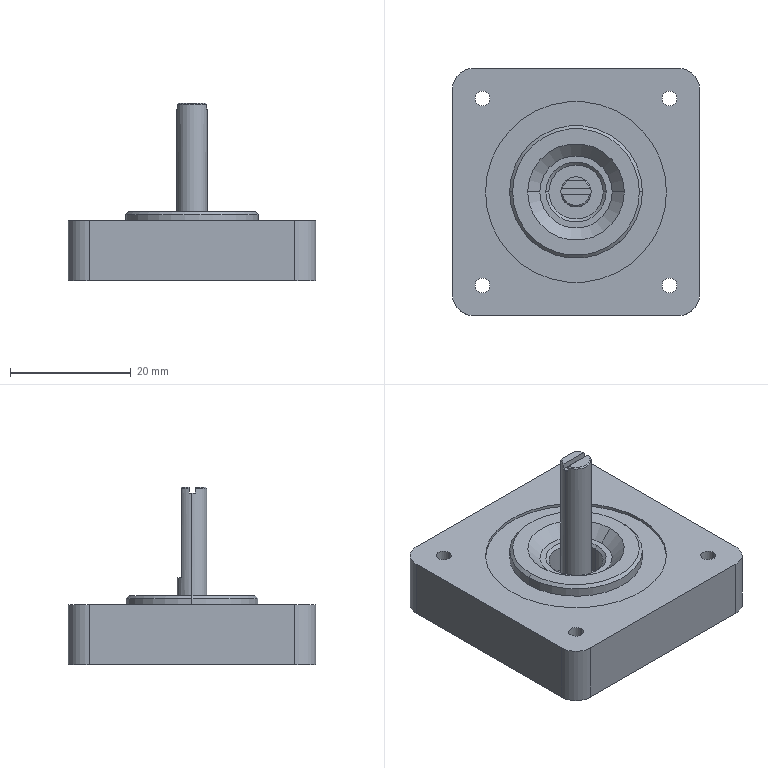Part | SolidWorks | features BaseBody 1 | 1 solid | 46 faces | box 41 x 41 x 29.5 mm | volume 16742 mm3 | cylinder 20 | plane 17 | cone 9 | commonest cylinder face diameters 2.459 x8 7 x4 5 x2 9 x2 22 x2 30 x2
STEP:
#1=CARTESIAN_POINT('',(-1.457,31.548,0.));
#2=VERTEX_POINT('',#1);
#3=CARTESIAN_POINT('',(-3.916,31.548,0.));
#4=VERTEX_POINT('',#3);
#5=CARTESIAN_POINT('',(-2.686,31.548,0.));
#6=DIRECTION('',(0.,0.,-1.));
#7=DIRECTION('',(1.,0.,0.));
#8=AXIS2_PLACEMENT_3D('',#5,#6,#7);
#9=CIRCLE('',#8,1.23);
#10=EDGE_CURVE('',#2,#4,#9,.T.);
#11=ORIENTED_EDGE('',*,*,#10,.T.);
#12=CARTESIAN_POINT('',(-3.916,31.548,10.));
#13=VERTEX_POINT('',#12);
#14=CARTESIAN_POINT('',(-3.916,31.548,-55.056));
#15=DIRECTION('',(0.,0.,1.));
#16=VECTOR('',#15,1000.);
#17=LINE('',#14,#16);
#18=EDGE_CURVE('',#4,#13,#17,.T.);
#19=ORIENTED_EDGE('',*,*,#18,.T.);
#20=CARTESIAN_POINT('',(-1.457,31.548,10.));
#21=VERTEX_POINT('',#20);
#22=CARTESIAN_POINT('',(-2.686,31.548,10.));
#23=DIRECTION('',(0.,0.,-1.));
#24=DIRECTION('',(1.,0.,0.));
#25=AXIS2_PLACEMENT_3D('',#22,#23,#24);
#26=CIRCLE('',#25,1.23);
#27=EDGE_CURVE('',#21,#13,#26,.T.);
#28=ORIENTED_EDGE('',*,*,#27,.F.);
#29=CARTESIAN_POINT('',(-1.457,31.548,-55.056));
#30=DIRECTION('',(0.,0.,1.));
#31=VECTOR('',#30,1000.);
#32=LINE('',#29,#31);
#33=EDGE_CURVE('',#2,#21,#32,.T.);
#34=ORIENTED_EDGE('',*,*,#33,.F.);
#35=EDGE_LOOP('',(#11,#19,#28,#34));
#36=FACE_OUTER_BOUND('',#35,.T.);
#37=CARTESIAN_POINT('',(-2.686,31.548,-55.056));
#38=DIRECTION('',(0.,0.,1.));
#39=DIRECTION('',(1.,0.,0.));
#40=AXIS2_PLACEMENT_3D('',#37,#38,#39);
#41=CYLINDRICAL_SURFACE('',#40,1.23);
#42=ADVANCED_FACE('',(#36),#41,.F.);
#43=CARTESIAN_POINT('',(-32.457,0.548,0.));
#44=VERTEX_POINT('',#43);
#45=CARTESIAN_POINT('',(-34.916,0.548,0.));
#46=VERTEX_POINT('',#45);
#47=CARTESIAN_POINT('',(-33.686,0.548,0.));
#48=DIRECTION('',(0.,0.,-1.));
#49=DIRECTION('',(1.,0.,0.));
#50=AXIS2_PLACEMENT_3D('',#47,#48,#49);
#51=CIRCLE('',#50,1.23);
#52=EDGE_CURVE('',#44,#46,#51,.T.);
#53=ORIENTED_EDGE('',*,*,#52,.T.);
#54=CARTESIAN_POINT('',(-34.916,0.548,10.));
#55=VERTEX_POINT('',#54);
#56=CARTESIAN_POINT('',(-34.916,0.548,-55.056));
#57=DIRECTION('',(0.,0.,1.));
#58=VECTOR('',#57,1000.);
#59=LINE('',#56,#58);
#60=EDGE_CURVE('',#46,#55,#59,.T.);
#61=ORIENTED_EDGE('',*,*,#60,.T.);
#62=CARTESIAN_POINT('',(-32.457,0.548,10.));
#63=VERTEX_POINT('',#62);
#64=CARTESIAN_POINT('',(-33.686,0.548,10.));
#65=DIRECTION('',(0.,0.,-1.));
#66=DIRECTION('',(1.,0.,0.));
#67=AXIS2_PLACEMENT_3D('',#64,#65,#66);
#68=CIRCLE('',#67,1.23);
#69=EDGE_CURVE('',#63,#55,#68,.T.);
#70=ORIENTED_EDGE('',*,*,#69,.F.);
#71=CARTESIAN_POINT('',(-32.457,0.548,-55.056));
#72=DIRECTION('',(0.,0.,1.));
#73=VECTOR('',#72,1000.);
#74=LINE('',#71,#73);
#75=EDGE_CURVE('',#44,#63,#74,.T.);
#76=ORIENTED_EDGE('',*,*,#75,.F.);
#77=EDGE_LOOP('',(#53,#61,#70,#76));
#78=FACE_OUTER_BOUND('',#77,.T.);
#79=CARTESIAN_POINT('',(-33.686,0.548,-55.056));
#80=DIRECTION('',(0.,0.,1.));
#81=DIRECTION('',(1.,0.,0.));
#82=AXIS2_PLACEMENT_3D('',#79,#80,#81);
#83=CYLINDRICAL_SURFACE('',#82,1.23);
#84=ADVANCED_FACE('',(#78),#83,.F.);
#85=CARTESIAN_POINT('',(-32.457,31.548,0.));
#86=VERTEX_POINT('',#85);
#87=CARTESIAN_POINT('',(-34.916,31.548,0.));
#88=VERTEX_POINT('',#87);
#89=CARTESIAN_POINT('',(-33.686,31.548,0.));
#90=DIRECTION('',(0.,0.,-1.));
#91=DIRECTION('',(1.,0.,0.));
#92=AXIS2_PLACEMENT_3D('',#89,#90,#91);
#93=CIRCLE('',#92,1.23);
#94=EDGE_CURVE('',#86,#88,#93,.T.);
#95=ORIENTED_EDGE('',*,*,#94,.T.);
#96=CARTESIAN_POINT('',(-34.916,31.548,10.));
#97=VERTEX_POINT('',#96);
#98=CARTESIAN_POINT('',(-34.916,31.548,-55.056));
#99=DIRECTION('',(0.,0.,1.));
#100=VECTOR('',#99,1000.);
#101=LINE('',#98,#100);
#102=EDGE_CURVE('',#88,#97,#101,.T.);
#103=ORIENTED_EDGE('',*,*,#102,.T.);
#104=CARTESIAN_POINT('',(-32.457,31.548,10.));
#105=VERTEX_POINT('',#104);
#106=CARTESIAN_POINT('',(-33.686,31.548,10.));
#107=DIRECTION('',(0.,0.,-1.));
#108=DIRECTION('',(1.,0.,0.));
#109=AXIS2_PLACEMENT_3D('',#106,#107,#108);
#110=CIRCLE('',#109,1.23);
#111=EDGE_CURVE('',#105,#97,#110,.T.);
#112=ORIENTED_EDGE('',*,*,#111,.F.);
#113=CARTESIAN_POINT('',(-32.457,31.548,-55.056));
#114=DIRECTION('',(0.,0.,1.));
#115=VECTOR('',#114,1000.);
#116=LINE('',#113,#115);
#117=EDGE_CURVE('',#86,#105,#116,.T.);
#118=ORIENTED_EDGE('',*,*,#117,.F.);
#119=EDGE_LOOP('',(#95,#103,#112,#118));
#120=FACE_OUTER_BOUND('',#119,.T.);
#121=CARTESIAN_POINT('',(-33.686,31.548,-55.056));
#122=DIRECTION('',(0.,0.,1.));
#123=DIRECTION('',(1.,0.,0.));
#124=AXIS2_PLACEMENT_3D('',#121,#122,#123);
#125=CYLINDRICAL_SURFACE('',#124,1.23);
#126=ADVANCED_FACE('',(#120),#125,.F.);
#127=CARTESIAN_POINT('',(-1.457,0.548,0.));
#128=VERTEX_POINT('',#127);
#129=CARTESIAN_POINT('',(-3.916,0.548,0.));
#130=VERTEX_POINT('',#129);
#131=CARTESIAN_POINT('',(-2.686,0.548,0.));
#132=DIRECTION('',(0.,0.,-1.));
#133=DIRECTION('',(1.,0.,0.));
#134=AXIS2_PLACEMENT_3D('',#131,#132,#133);
#135=CIRCLE('',#134,1.23);
#136=EDGE_CURVE('',#128,#130,#135,.T.);
#137=ORIENTED_EDGE('',*,*,#136,.T.);
#138=CARTESIAN_POINT('',(-3.916,0.548,10.));
#139=VERTEX_POINT('',#138);
#140=CARTESIAN_POINT('',(-3.916,0.548,-55.056));
#141=DIRECTION('',(0.,0.,1.));
#142=VECTOR('',#141,1000.);
#143=LINE('',#140,#142);
#144=EDGE_CURVE('',#130,#139,#143,.T.);
#145=ORIENTED_EDGE('',*,*,#144,.T.);
#146=CARTESIAN_POINT('',(-1.457,0.548,10.));
#147=VERTEX_POINT('',#146);
#148=CARTESIAN_POINT('',(-2.686,0.548,10.));
#149=DIRECTION('',(0.,0.,-1.));
#150=DIRECTION('',(1.,0.,0.));
#151=AXIS2_PLACEMENT_3D('',#148,#149,#150);
#152=CIRCLE('',#151,1.23);
#153=EDGE_CURVE('',#147,#139,#152,.T.);
#154=ORIENTED_EDGE('',*,*,#153,.F.);
#155=CARTESIAN_POINT('',(-1.457,0.548,-55.056));
#156=DIRECTION('',(0.,0.,1.));
#157=VECTOR('',#156,1000.);
#158=LINE('',#155,#157);
#159=EDGE_CURVE('',#128,#147,#158,.T.);
#160=ORIENTED_EDGE('',*,*,#159,.F.);
#161=EDGE_LOOP('',(#137,#145,#154,#160));
#162=FACE_OUTER_BOUND('',#161,.T.);
#163=CARTESIAN_POINT('',(-2.686,0.548,-55.056));
#164=DIRECTION('',(0.,0.,1.));
#165=DIRECTION('',(1.,0.,0.));
#166=AXIS2_PLACEMENT_3D('',#163,#164,#165);
#167=CYLINDRICAL_SURFACE('',#166,1.23);
#168=ADVANCED_FACE('',(#162),#167,.F.);
#169=CARTESIAN_POINT('',(-3.186,16.048,10.));
#170=VERTEX_POINT('',#169);
#171=CARTESIAN_POINT('',(-33.186,16.048,10.));
#172=VERTEX_POINT('',#171);
#173=CARTESIAN_POINT('',(-18.186,16.048,10.));
#174=DIRECTION('',(0.,0.,-1.));
#175=DIRECTION('',(-1.,0.,0.));
#176=AXIS2_PLACEMENT_3D('',#173,#174,#175);
#177=CIRCLE('',#176,15.);
#178=EDGE_CURVE('',#170,#172,#177,.T.);
#179=ORIENTED_EDGE('',*,*,#178,.F.);
#180=CARTESIAN_POINT('',(-3.186,16.048,9.5));
#181=VERTEX_POINT('',#180);
#182=CARTESIAN_POINT('',(-3.186,16.048,10.));
#183=DIRECTION('',(0.,0.,-1.));
#184=VECTOR('',#183,1000.);
#185=LINE('',#182,#184);
#186=EDGE_CURVE('',#170,#181,#185,.T.);
#187=ORIENTED_EDGE('',*,*,#186,.T.);
#188=CARTESIAN_POINT('',(-33.186,16.048,9.5));
#189=VERTEX_POINT('',#188);
#190=CARTESIAN_POINT('',(-18.186,16.048,9.5));
#191=DIRECTION('',(0.,0.,1.));
#192=DIRECTION('',(-1.,0.,0.));
#193=AXIS2_PLACEMENT_3D('',#190,#191,#192);
#194=CIRCLE('',#193,15.);
#195=EDGE_CURVE('',#189,#181,#194,.T.);
#196=ORIENTED_EDGE('',*,*,#195,.F.);
#197=CARTESIAN_POINT('',(-33.186,16.048,10.));
#198=DIRECTION('',(0.,0.,-1.));
#199=VECTOR('',#198,1000.);
#200=LINE('',#197,#199);
#201=EDGE_CURVE('',#172,#189,#200,.T.);
#202=ORIENTED_EDGE('',*,*,#201,.F.);
#203=EDGE_LOOP('',(#179,#187,#196,#202));
#204=FACE_OUTER_BOUND('',#203,.T.);
#205=CARTESIAN_POINT('',(-18.186,16.048,10.));
#206=DIRECTION('',(0.,0.,-1.));
#207=DIRECTION('',(-1.,0.,0.));
#208=AXIS2_PLACEMENT_3D('',#205,#206,#207);
#209=CYLINDRICAL_SURFACE('',#208,15.);
#210=ADVANCED_FACE('',(#204),#209,.F.);
#211=CARTESIAN_POINT('',(-7.186,16.048,9.5));
#212=VERTEX_POINT('',#211);
#213=CARTESIAN_POINT('',(-29.186,16.048,9.5));
#214=VERTEX_POINT('',#213);
#215=CARTESIAN_POINT('',(-18.186,16.048,9.5));
#216=DIRECTION('',(0.,0.,1.));
#217=DIRECTION('',(1.,0.,0.));
#218=AXIS2_PLACEMENT_3D('',#215,#216,#217);
#219=CIRCLE('',#218,11.);
#220=EDGE_CURVE('',#212,#214,#219,.T.);
#221=ORIENTED_EDGE('',*,*,#220,.T.);
#222=CARTESIAN_POINT('',(-29.186,16.048,11.));
#223=VERTEX_POINT('',#222);
#224=CARTESIAN_POINT('',(-29.186,16.048,9.5));
#225=DIRECTION('',(0.,0.,1.));
#226=VECTOR('',#225,1000.);
#227=LINE('',#224,#226);
#228=EDGE_CURVE('',#214,#223,#227,.T.);
#229=ORIENTED_EDGE('',*,*,#228,.T.);
#230=CARTESIAN_POINT('',(-7.186,16.048,11.));
#231=VERTEX_POINT('',#230);
#232=CARTESIAN_POINT('',(-18.186,16.048,11.));
#233=DIRECTION('',(0.,0.,-1.));
#234=DIRECTION('',(1.,0.,0.));
#235=AXIS2_PLACEMENT_3D('',#232,#233,#234);
#236=CIRCLE('',#235,11.);
#237=EDGE_CURVE('',#223,#231,#236,.T.);
#238=ORIENTED_EDGE('',*,*,#237,.T.);
#239=CARTESIAN_POINT('',(-7.186,16.048,9.5));
#240=DIRECTION('',(0.,0.,1.));
#241=VECTOR('',#240,1000.);
#242=LINE('',#239,#241);
#243=EDGE_CURVE('',#212,#231,#242,.T.);
#244=ORIENTED_EDGE('',*,*,#243,.F.);
#245=EDGE_LOOP('',(#221,#229,#238,#244));
#246=FACE_OUTER_BOUND('',#245,.T.);
#247=CARTESIAN_POINT('',(-18.186,16.048,9.5));
#248=DIRECTION('',(0.,0.,1.));
#249=DIRECTION('',(1.,0.,0.));
#250=AXIS2_PLACEMENT_3D('',#247,#248,#249);
#251=CYLINDRICAL_SURFACE('',#250,11.);
#252=ADVANCED_FACE('',(#246),#251,.T.);
#253=CARTESIAN_POINT('',(-28.686,16.048,11.5));
#254=VERTEX_POINT('',#253);
#255=CARTESIAN_POINT('',(-7.686,16.048,11.5));
#256=VERTEX_POINT('',#255);
#257=CARTESIAN_POINT('',(-18.186,16.048,11.5));
#258=DIRECTION('',(0.,0.,-1.));
#259=DIRECTION('',(-1.,0.,0.));
#260=AXIS2_PLACEMENT_3D('',#257,#258,#259);
#261=CIRCLE('',#260,10.5);
#262=EDGE_CURVE('',#254,#256,#261,.T.);
#263=ORIENTED_EDGE('',*,*,#262,.T.);
#264=CARTESIAN_POINT('',(-7.186,16.048,11.));
#265=DIRECTION('',(0.7071,0.,-0.7071));
#266=VECTOR('',#265,1000.);
#267=LINE('',#264,#266);
#268=EDGE_CURVE('',#256,#231,#267,.T.);
#269=ORIENTED_EDGE('',*,*,#268,.T.);
#270=ORIENTED_EDGE('',*,*,#237,.F.);
#271=CARTESIAN_POINT('',(-29.186,16.048,11.));
#272=DIRECTION('',(-0.7071,0.,-0.7071));
#273=VECTOR('',#272,1000.);
#274=LINE('',#271,#273);
#275=EDGE_CURVE('',#254,#223,#274,.T.);
#276=ORIENTED_EDGE('',*,*,#275,.F.);
#277=EDGE_LOOP('',(#263,#269,#270,#276));
#278=FACE_OUTER_BOUND('',#277,.T.);
#279=CARTESIAN_POINT('',(-18.186,16.048,11.));
#280=DIRECTION('',(0.,0.,-1.));
#281=DIRECTION('',(-1.,0.,0.));
#282=AXIS2_PLACEMENT_3D('',#279,#280,#281);
#283=CONICAL_SURFACE('',#282,11.,0.7854);
#284=ADVANCED_FACE('',(#278),#283,.T.);
#285=CARTESIAN_POINT('',(-24.186,16.048,9.5));
#286=VERTEX_POINT('',#285);
#287=CARTESIAN_POINT('',(-12.186,16.048,9.5));
#288=VERTEX_POINT('',#287);
#289=CARTESIAN_POINT('',(-18.186,16.048,9.5));
#290=DIRECTION('',(0.,0.,1.));
#291=DIRECTION('',(1.,0.,0.));
#292=AXIS2_PLACEMENT_3D('',#289,#290,#291);
#293=CIRCLE('',#292,6.);
#294=EDGE_CURVE('',#286,#288,#293,.T.);
#295=ORIENTED_EDGE('',*,*,#294,.F.);
#296=CARTESIAN_POINT('',(-26.186,16.048,11.5));
#297=VERTEX_POINT('',#296);
#298=CARTESIAN_POINT('',(-26.186,16.048,11.5));
#299=DIRECTION('',(-0.7071,0.,0.7071));
#300=VECTOR('',#299,1000.);
#301=LINE('',#298,#300);
#302=EDGE_CURVE('',#286,#297,#301,.T.);
#303=ORIENTED_EDGE('',*,*,#302,.T.);
#304=CARTESIAN_POINT('',(-10.186,16.048,11.5));
#305=VERTEX_POINT('',#304);
#306=CARTESIAN_POINT('',(-18.186,16.048,11.5));
#307=DIRECTION('',(0.,0.,1.));
#308=DIRECTION('',(1.,0.,0.));
#309=AXIS2_PLACEMENT_3D('',#306,#307,#308);
#310=CIRCLE('',#309,8.);
#311=EDGE_CURVE('',#297,#305,#310,.T.);
#312=ORIENTED_EDGE('',*,*,#311,.T.);
#313=CARTESIAN_POINT('',(-10.186,16.048,11.5));
#314=DIRECTION('',(0.7071,0.,0.7071));
#315=VECTOR('',#314,1000.);
#316=LINE('',#313,#315);
#317=EDGE_CURVE('',#288,#305,#316,.T.);
#318=ORIENTED_EDGE('',*,*,#317,.F.);
#319=EDGE_LOOP('',(#295,#303,#312,#318));
#320=FACE_OUTER_BOUND('',#319,.T.);
#321=CARTESIAN_POINT('',(-18.186,16.048,11.5));
#322=DIRECTION('',(0.,0.,1.));
#323=DIRECTION('',(1.,0.,0.));
#324=AXIS2_PLACEMENT_3D('',#321,#322,#323);
#325=CONICAL_SURFACE('',#324,8.,0.7854);
#326=ADVANCED_FACE('',(#320),#325,.F.);
#327=CARTESIAN_POINT('',(-22.686,16.048,9.));
#328=VERTEX_POINT('',#327);
#329=CARTESIAN_POINT('',(-13.686,16.048,9.));
#330=VERTEX_POINT('',#329);
#331=CARTESIAN_POINT('',(-18.186,16.048,9.));
#332=DIRECTION('',(0.,0.,1.));
#333=DIRECTION('',(-1.,0.,0.));
#334=AXIS2_PLACEMENT_3D('',#331,#332,#333);
#335=CIRCLE('',#334,4.5);
#336=EDGE_CURVE('',#328,#330,#335,.T.);
#337=ORIENTED_EDGE('',*,*,#336,.F.);
#338=CARTESIAN_POINT('',(-23.186,16.048,9.5));
#339=VERTEX_POINT('',#338);
#340=CARTESIAN_POINT('',(-23.186,16.048,9.5));
#341=DIRECTION('',(-0.7071,0.,0.7071));
#342=VECTOR('',#341,1000.);
#343=LINE('',#340,#342);
#344=EDGE_CURVE('',#328,#339,#343,.T.);
#345=ORIENTED_EDGE('',*,*,#344,.T.);
#346=CARTESIAN_POINT('',(-13.186,16.048,9.5));
#347=VERTEX_POINT('',#346);
#348=CARTESIAN_POINT('',(-18.186,16.048,9.5));
#349=DIRECTION('',(0.,0.,1.));
#350=DIRECTION('',(1.,0.,0.));
#351=AXIS2_PLACEMENT_3D('',#348,#349,#350);
#352=CIRCLE('',#351,5.);
#353=EDGE_CURVE('',#339,#347,#352,.T.);
#354=ORIENTED_EDGE('',*,*,#353,.T.);
#355=CARTESIAN_POINT('',(-13.186,16.048,9.5));
#356=DIRECTION('',(0.7071,0.,0.7071));
#357=VECTOR('',#356,1000.);
#358=LINE('',#355,#357);
#359=EDGE_CURVE('',#330,#347,#358,.T.);
#360=ORIENTED_EDGE('',*,*,#359,.F.);
#361=EDGE_LOOP('',(#337,#345,#354,#360));
#362=FACE_OUTER_BOUND('',#361,.T.);
#363=CARTESIAN_POINT('',(-18.186,16.048,9.5));
#364=DIRECTION('',(0.,0.,1.));
#365=DIRECTION('',(1.,0.,0.));
#366=AXIS2_PLACEMENT_3D('',#363,#364,#365);
#367=CONICAL_SURFACE('',#366,5.,0.7854);
#368=ADVANCED_FACE('',(#362),#367,.F.);
#369=CARTESIAN_POINT('',(-22.686,16.048,4.5));
#370=VERTEX_POINT('',#369);
#371=CARTESIAN_POINT('',(-13.686,16.048,4.5));
#372=VERTEX_POINT('',#371);
#373=CARTESIAN_POINT('',(-18.186,16.048,4.5));
#374=DIRECTION('',(0.,0.,1.));
#375=DIRECTION('',(1.,0.,0.));
#376=AXIS2_PLACEMENT_3D('',#373,#374,#375);
#377=CIRCLE('',#376,4.5);
#378=EDGE_CURVE('',#370,#372,#377,.T.);
#379=ORIENTED_EDGE('',*,*,#378,.F.);
#380=CARTESIAN_POINT('',(-22.686,16.048,7.));
#381=DIRECTION('',(0.,0.,1.));
#382=VECTOR('',#381,1000.);
#383=LINE('',#380,#382);
#384=EDGE_CURVE('',#370,#328,#383,.T.);
#385=ORIENTED_EDGE('',*,*,#384,.T.);
#386=ORIENTED_EDGE('',*,*,#336,.T.);
#387=CARTESIAN_POINT('',(-13.686,16.048,7.));
#388=DIRECTION('',(0.,0.,1.));
#389=VECTOR('',#388,1000.);
#390=LINE('',#387,#389);
#391=EDGE_CURVE('',#372,#330,#390,.T.);
#392=ORIENTED_EDGE('',*,*,#391,.F.);
#393=EDGE_LOOP('',(#379,#385,#386,#392));
#394=FACE_OUTER_BOUND('',#393,.T.);
#395=CARTESIAN_POINT('',(-18.186,16.048,7.));
#396=DIRECTION('',(0.,0.,1.));
#397=DIRECTION('',(1.,0.,0.));
#398=AXIS2_PLACEMENT_3D('',#395,#396,#397);
#399=CYLINDRICAL_SURFACE('',#398,4.5);
#400=ADVANCED_FACE('',(#394),#399,.F.);
#401=CARTESIAN_POINT('',(-20.686,16.048,4.5));
#402=VERTEX_POINT('',#401);
#403=CARTESIAN_POINT('',(-15.686,16.048,4.5));
#404=VERTEX_POINT('',#403);
#405=CARTESIAN_POINT('',(-18.186,16.048,4.5));
#406=DIRECTION('',(0.,0.,-1.));
#407=DIRECTION('',(1.,0.,0.));
#408=AXIS2_PLACEMENT_3D('',#405,#406,#407);
#409=CIRCLE('',#408,2.5);
#410=EDGE_CURVE('',#402,#404,#409,.T.);
#411=ORIENTED_EDGE('',*,*,#410,.F.);
#412=CARTESIAN_POINT('',(-20.686,16.048,28.5));
#413=VERTEX_POINT('',#412);
#414=CARTESIAN_POINT('',(-20.686,16.048,4.5));
#415=DIRECTION('',(0.,0.,1.));
#416=VECTOR('',#415,1000.);
#417=LINE('',#414,#416);
#418=EDGE_CURVE('',#402,#413,#417,.T.);
#419=ORIENTED_EDGE('',*,*,#418,.T.);
#420=CARTESIAN_POINT('',(-20.637,16.545,28.5));
#421=VERTEX_POINT('',#420);
#422=CARTESIAN_POINT('',(-18.186,16.048,28.5));
#423=DIRECTION('',(0.,0.,1.));
#424=DIRECTION('',(1.,0.,0.));
#425=AXIS2_PLACEMENT_3D('',#422,#423,#424);
#426=CIRCLE('',#425,2.5);
#427=EDGE_CURVE('',#421,#413,#426,.T.);
#428=ORIENTED_EDGE('',*,*,#427,.F.);
#429=CARTESIAN_POINT('',(-20.637,16.545,29.3));
#430=VERTEX_POINT('',#429);
#431=CARTESIAN_POINT('',(-20.637,16.545,29.5));
#432=DIRECTION('',(0.,0.,1.));
#433=VECTOR('',#432,1000.);
#434=LINE('',#431,#433);
#435=EDGE_CURVE('',#421,#430,#434,.T.);
#436=ORIENTED_EDGE('',*,*,#435,.T.);
#437=CARTESIAN_POINT('',(-19.921,17.848,29.3));
#438=VERTEX_POINT('',#437);
#439=CARTESIAN_POINT('',(-18.186,16.048,29.3));
#440=DIRECTION('',(0.,0.,-1.));
#441=DIRECTION('',(1.,0.,0.));
#442=AXIS2_PLACEMENT_3D('',#439,#440,#441);
#443=CIRCLE('',#442,2.5);
#444=EDGE_CURVE('',#430,#438,#443,.T.);
#445=ORIENTED_EDGE('',*,*,#444,.T.);
#446=CARTESIAN_POINT('',(-19.921,17.848,14.5));
#447=VERTEX_POINT('',#446);
#448=CARTESIAN_POINT('',(-19.921,17.848,4.5));
#449=DIRECTION('',(0.,0.,-1.));
#450=VECTOR('',#449,1000.);
#451=LINE('',#448,#450);
#452=EDGE_CURVE('',#438,#447,#451,.T.);
#453=ORIENTED_EDGE('',*,*,#452,.T.);
#454=CARTESIAN_POINT('',(-16.451,17.848,14.5));
#455=VERTEX_POINT('',#454);
#456=CARTESIAN_POINT('',(-18.186,16.048,14.5));
#457=DIRECTION('',(0.,0.,-1.));
#458=DIRECTION('',(1.,0.,0.));
#459=AXIS2_PLACEMENT_3D('',#456,#457,#458);
#460=CIRCLE('',#459,2.5);
#461=EDGE_CURVE('',#447,#455,#460,.T.);
#462=ORIENTED_EDGE('',*,*,#461,.T.);
#463=CARTESIAN_POINT('',(-16.451,17.848,29.3));
#464=VERTEX_POINT('',#463);
#465=CARTESIAN_POINT('',(-16.451,17.848,4.5));
#466=DIRECTION('',(0.,0.,1.));
#467=VECTOR('',#466,1000.);
#468=LINE('',#465,#467);
#469=EDGE_CURVE('',#455,#464,#468,.T.);
#470=ORIENTED_EDGE('',*,*,#469,.T.);
#471=CARTESIAN_POINT('',(-15.736,16.545,29.3));
#472=VERTEX_POINT('',#471);
#473=CARTESIAN_POINT('',(-18.186,16.048,29.3));
#474=DIRECTION('',(0.,0.,-1.));
#475=DIRECTION('',(1.,0.,0.));
#476=AXIS2_PLACEMENT_3D('',#473,#474,#475);
#477=CIRCLE('',#476,2.5);
#478=EDGE_CURVE('',#464,#472,#477,.T.);
#479=ORIENTED_EDGE('',*,*,#478,.T.);
#480=CARTESIAN_POINT('',(-15.736,16.545,28.5));
#481=VERTEX_POINT('',#480);
#482=CARTESIAN_POINT('',(-15.736,16.545,29.5));
#483=DIRECTION('',(0.,0.,-1.));
#484=VECTOR('',#483,1000.);
#485=LINE('',#482,#484);
#486=EDGE_CURVE('',#472,#481,#485,.T.);
#487=ORIENTED_EDGE('',*,*,#486,.T.);
#488=CARTESIAN_POINT('',(-15.686,16.048,28.5));
#489=VERTEX_POINT('',#488);
#490=CARTESIAN_POINT('',(-18.186,16.048,28.5));
#491=DIRECTION('',(0.,0.,1.));
#492=DIRECTION('',(1.,0.,0.));
#493=AXIS2_PLACEMENT_3D('',#490,#491,#492);
#494=CIRCLE('',#493,2.5);
#495=EDGE_CURVE('',#489,#481,#494,.T.);
#496=ORIENTED_EDGE('',*,*,#495,.F.);
#497=CARTESIAN_POINT('',(-15.686,16.048,4.5));
#498=DIRECTION('',(0.,0.,1.));
#499=VECTOR('',#498,1000.);
#500=LINE('',#497,#499);
#501=EDGE_CURVE('',#404,#489,#500,.T.);
#502=ORIENTED_EDGE('',*,*,#501,.F.);
#503=EDGE_LOOP('',(#411,#419,#428,#436,#445,#453,#462,#470,#479,#487,#496,#502));
#504=FACE_OUTER_BOUND('',#503,.T.);
#505=CARTESIAN_POINT('',(-18.186,16.048,4.5));
#506=DIRECTION('',(0.,0.,1.));
#507=DIRECTION('',(1.,0.,0.));
#508=AXIS2_PLACEMENT_3D('',#505,#506,#507);
#509=CYLINDRICAL_SURFACE('',#508,2.5);
#510=ADVANCED_FACE('',(#504),#509,.T.);
#511=ORIENTED_EDGE('',*,*,#10,.F.);
#512=CARTESIAN_POINT('',(-2.686,31.548,0.));
#513=DIRECTION('',(0.,0.,-1.));
#514=DIRECTION('',(1.,0.,0.));
#515=AXIS2_PLACEMENT_3D('',#512,#513,#514);
#516=CIRCLE('',#515,1.23);
#517=EDGE_CURVE('',#4,#2,#516,.T.);
#518=ORIENTED_EDGE('',*,*,#517,.F.);
#519=EDGE_LOOP('',(#511,#518));
#520=FACE_BOUND('',#519,.T.);
#521=ORIENTED_EDGE('',*,*,#52,.F.);
#522=CARTESIAN_POINT('',(-33.686,0.548,0.));
#523=DIRECTION('',(0.,0.,-1.));
#524=DIRECTION('',(1.,0.,0.));
#525=AXIS2_PLACEMENT_3D('',#522,#523,#524);
#526=CIRCLE('',#525,1.23);
#527=EDGE_CURVE('',#46,#44,#526,.T.);
#528=ORIENTED_EDGE('',*,*,#527,.F.);
#529=EDGE_LOOP('',(#521,#528));
#530=FACE_BOUND('',#529,.T.);
#531=ORIENTED_EDGE('',*,*,#94,.F.);
#532=CARTESIAN_POINT('',(-33.686,31.548,0.));
#533=DIRECTION('',(0.,0.,-1.));
#534=DIRECTION('',(1.,0.,0.));
#535=AXIS2_PLACEMENT_3D('',#532,#533,#534);
#536=CIRCLE('',#535,1.23);
#537=EDGE_CURVE('',#88,#86,#536,.T.);
#538=ORIENTED_EDGE('',*,*,#537,.F.);
#539=EDGE_LOOP('',(#531,#538));
#540=FACE_BOUND('',#539,.T.);
#541=ORIENTED_EDGE('',*,*,#136,.F.);
#542=CARTESIAN_POINT('',(-2.686,0.548,0.));
#543=DIRECTION('',(0.,0.,-1.));
#544=DIRECTION('',(1.,0.,0.));
#545=AXIS2_PLACEMENT_3D('',#542,#543,#544);
#546=CIRCLE('',#545,1.23);
#547=EDGE_CURVE('',#130,#128,#546,.T.);
#548=ORIENTED_EDGE('',*,*,#547,.F.);
#549=EDGE_LOOP('',(#541,#548));
#550=FACE_BOUND('',#549,.T.);
#551=CARTESIAN_POINT('',(-38.686,33.048,0.));
#552=VERTEX_POINT('',#551);
#553=CARTESIAN_POINT('',(-38.686,-0.952,0.));
#554=VERTEX_POINT('',#553);
#555=CARTESIAN_POINT('',(-38.686,16.048,0.));
#556=DIRECTION('',(0.,-1.,0.));
#557=VECTOR('',#556,1000.);
#558=LINE('',#555,#557);
#559=EDGE_CURVE('',#552,#554,#558,.T.);
#560=ORIENTED_EDGE('',*,*,#559,.F.);
#561=CARTESIAN_POINT('',(-35.186,36.548,0.));
#562=VERTEX_POINT('',#561);
#563=CARTESIAN_POINT('',(-35.186,33.048,0.));
#564=DIRECTION('',(0.,0.,1.));
#565=DIRECTION('',(1.,0.,0.));
#566=AXIS2_PLACEMENT_3D('',#563,#564,#565);
#567=CIRCLE('',#566,3.5);
#568=EDGE_CURVE('',#562,#552,#567,.T.);
#569=ORIENTED_EDGE('',*,*,#568,.F.);
#570=CARTESIAN_POINT('',(-1.186,36.548,0.));
#571=VERTEX_POINT('',#570);
#572=CARTESIAN_POINT('',(-18.186,36.548,0.));
#573=DIRECTION('',(-1.,0.,0.));
#574=VECTOR('',#573,1000.);
#575=LINE('',#572,#574);
#576=EDGE_CURVE('',#571,#562,#575,.T.);
#577=ORIENTED_EDGE('',*,*,#576,.F.);
#578=CARTESIAN_POINT('',(2.314,33.048,0.));
#579=VERTEX_POINT('',#578);
#580=CARTESIAN_POINT('',(-1.186,33.048,0.));
#581=DIRECTION('',(0.,0.,1.));
#582=DIRECTION('',(1.,0.,0.));
#583=AXIS2_PLACEMENT_3D('',#580,#581,#582);
#584=CIRCLE('',#583,3.5);
#585=EDGE_CURVE('',#579,#571,#584,.T.);
#586=ORIENTED_EDGE('',*,*,#585,.F.);
#587=CARTESIAN_POINT('',(2.314,-0.952,0.));
#588=VERTEX_POINT('',#587);
#589=CARTESIAN_POINT('',(2.314,16.048,0.));
#590=DIRECTION('',(0.,1.,0.));
#591=VECTOR('',#590,1000.);
#592=LINE('',#589,#591);
#593=EDGE_CURVE('',#588,#579,#592,.T.);
#594=ORIENTED_EDGE('',*,*,#593,.F.);
#595=CARTESIAN_POINT('',(-1.186,-4.452,0.));
#596=VERTEX_POINT('',#595);
#597=CARTESIAN_POINT('',(-1.186,-0.952,0.));
#598=DIRECTION('',(0.,0.,1.));
#599=DIRECTION('',(1.,0.,0.));
#600=AXIS2_PLACEMENT_3D('',#597,#598,#599);
#601=CIRCLE('',#600,3.5);
#602=EDGE_CURVE('',#596,#588,#601,.T.);
#603=ORIENTED_EDGE('',*,*,#602,.F.);
#604=CARTESIAN_POINT('',(-35.186,-4.452,0.));
#605=VERTEX_POINT('',#604);
#606=CARTESIAN_POINT('',(-18.186,-4.452,0.));
#607=DIRECTION('',(1.,0.,0.));
#608=VECTOR('',#607,1000.);
#609=LINE('',#606,#608);
#610=EDGE_CURVE('',#605,#596,#609,.T.);
#611=ORIENTED_EDGE('',*,*,#610,.F.);
#612=CARTESIAN_POINT('',(-35.186,-0.952,0.));
#613=DIRECTION('',(0.,0.,1.));
#614=DIRECTION('',(1.,0.,0.));
#615=AXIS2_PLACEMENT_3D('',#612,#613,#614);
#616=CIRCLE('',#615,3.5);
#617=EDGE_CURVE('',#554,#605,#616,.T.);
#618=ORIENTED_EDGE('',*,*,#617,.F.);
#619=EDGE_LOOP('',(#560,#569,#577,#586,#594,#603,#611,#618));
#620=FACE_OUTER_BOUND('',#619,.T.);
#621=CARTESIAN_POINT('',(-18.186,16.048,0.));
#622=DIRECTION('',(0.,0.,1.));
#623=DIRECTION('',(1.,0.,0.));
#624=AXIS2_PLACEMENT_3D('',#621,#622,#623);
#625=PLANE('',#624);
#626=ADVANCED_FACE('',(#520,#530,#540,#550,#620),#625,.F.);
#627=ORIENTED_EDGE('',*,*,#18,.F.);
#628=ORIENTED_EDGE('',*,*,#517,.T.);
#629=ORIENTED_EDGE('',*,*,#33,.T.);
#630=CARTESIAN_POINT('',(-2.686,31.548,10.));
#631=DIRECTION('',(0.,0.,-1.));
#632=DIRECTION('',(1.,0.,0.));
#633=AXIS2_PLACEMENT_3D('',#630,#631,#632);
#634=CIRCLE('',#633,1.23);
#635=EDGE_CURVE('',#13,#21,#634,.T.);
#636=ORIENTED_EDGE('',*,*,#635,.F.);
#637=EDGE_LOOP('',(#627,#628,#629,#636));
#638=FACE_OUTER_BOUND('',#637,.T.);
#639=CARTESIAN_POINT('',(-2.686,31.548,-55.056));
#640=DIRECTION('',(0.,0.,1.));
#641=DIRECTION('',(1.,0.,0.));
#642=AXIS2_PLACEMENT_3D('',#639,#640,#641);
#643=CYLINDRICAL_SURFACE('',#642,1.23);
#644=ADVANCED_FACE('',(#638),#643,.F.);
#645=ORIENTED_EDGE('',*,*,#60,.F.);
#646=ORIENTED_EDGE('',*,*,#527,.T.);
#647=ORIENTED_EDGE('',*,*,#75,.T.);
#648=CARTESIAN_POINT('',(-33.686,0.548,10.));
#649=DIRECTION('',(0.,0.,-1.));
#650=DIRECTION('',(1.,0.,0.));
#651=AXIS2_PLACEMENT_3D('',#648,#649,#650);
#652=CIRCLE('',#651,1.23);
#653=EDGE_CURVE('',#55,#63,#652,.T.);
#654=ORIENTED_EDGE('',*,*,#653,.F.);
#655=EDGE_LOOP('',(#645,#646,#647,#654));
#656=FACE_OUTER_BOUND('',#655,.T.);
#657=CARTESIAN_POINT('',(-33.686,0.548,-55.056));
#658=DIRECTION('',(0.,0.,1.));
#659=DIRECTION('',(1.,0.,0.));
#660=AXIS2_PLACEMENT_3D('',#657,#658,#659);
#661=CYLINDRICAL_SURFACE('',#660,1.23);
#662=ADVANCED_FACE('',(#656),#661,.F.);
#663=ORIENTED_EDGE('',*,*,#102,.F.);
#664=ORIENTED_EDGE('',*,*,#537,.T.);
#665=ORIENTED_EDGE('',*,*,#117,.T.);
#666=CARTESIAN_POINT('',(-33.686,31.548,10.));
#667=DIRECTION('',(0.,0.,-1.));
#668=DIRECTION('',(1.,0.,0.));
#669=AXIS2_PLACEMENT_3D('',#666,#667,#668);
#670=CIRCLE('',#669,1.23);
#671=EDGE_CURVE('',#97,#105,#670,.T.);
#672=ORIENTED_EDGE('',*,*,#671,.F.);
#673=EDGE_LOOP('',(#663,#664,#665,#672));
#674=FACE_OUTER_BOUND('',#673,.T.);
#675=CARTESIAN_POINT('',(-33.686,31.548,-55.056));
#676=DIRECTION('',(0.,0.,1.));
#677=DIRECTION('',(1.,0.,0.));
#678=AXIS2_PLACEMENT_3D('',#675,#676,#677);
#679=CYLINDRICAL_SURFACE('',#678,1.23);
#680=ADVANCED_FACE('',(#674),#679,.F.);
#681=ORIENTED_EDGE('',*,*,#144,.F.);
#682=ORIENTED_EDGE('',*,*,#547,.T.);
#683=ORIENTED_EDGE('',*,*,#159,.T.);
#684=CARTESIAN_POINT('',(-2.686,0.548,10.));
#685=DIRECTION('',(0.,0.,-1.));
#686=DIRECTION('',(1.,0.,0.));
#687=AXIS2_PLACEMENT_3D('',#684,#685,#686);
#688=CIRCLE('',#687,1.23);
#689=EDGE_CURVE('',#139,#147,#688,.T.);
#690=ORIENTED_EDGE('',*,*,#689,.F.);
#691=EDGE_LOOP('',(#681,#682,#683,#690));
#692=FACE_OUTER_BOUND('',#691,.T.);
#693=CARTESIAN_POINT('',(-2.686,0.548,-55.056));
#694=DIRECTION('',(0.,0.,1.));
#695=DIRECTION('',(1.,0.,0.));
#696=AXIS2_PLACEMENT_3D('',#693,#694,#695);
#697=CYLINDRICAL_SURFACE('',#696,1.23);
#698=ADVANCED_FACE('',(#692),#697,.F.);
#699=ORIENTED_EDGE('',*,*,#617,.T.);
#700=CARTESIAN_POINT('',(-35.186,-4.452,10.));
#701=VERTEX_POINT('',#700);
#702=CARTESIAN_POINT('',(-35.186,-4.452,0.));
#703=DIRECTION('',(0.,0.,1.));
#704=VECTOR('',#703,1000.);
#705=LINE('',#702,#704);
#706=EDGE_CURVE('',#605,#701,#705,.T.);
#707=ORIENTED_EDGE('',*,*,#706,.T.);
#708=CARTESIAN_POINT('',(-38.686,-0.952,10.));
#709=VERTEX_POINT('',#708);
#710=CARTESIAN_POINT('',(-35.186,-0.952,10.));
#711=DIRECTION('',(0.,0.,-1.));
#712=DIRECTION('',(1.,0.,0.));
#713=AXIS2_PLACEMENT_3D('',#710,#711,#712);
#714=CIRCLE('',#713,3.5);
#715=EDGE_CURVE('',#701,#709,#714,.T.);
#716=ORIENTED_EDGE('',*,*,#715,.T.);
#717=CARTESIAN_POINT('',(-38.686,-0.952,0.));
#718=DIRECTION('',(0.,0.,-1.));
#719=VECTOR('',#718,1000.);
#720=LINE('',#717,#719);
#721=EDGE_CURVE('',#709,#554,#720,.T.);
#722=ORIENTED_EDGE('',*,*,#721,.T.);
#723=EDGE_LOOP('',(#699,#707,#716,#722));
#724=FACE_OUTER_BOUND('',#723,.T.);
#725=CARTESIAN_POINT('',(-35.186,-0.952,0.));
#726=DIRECTION('',(0.,0.,1.));
#727=DIRECTION('',(1.,0.,0.));
#728=AXIS2_PLACEMENT_3D('',#725,#726,#727);
#729=CYLINDRICAL_SURFACE('',#728,3.5);
#730=ADVANCED_FACE('',(#724),#729,.T.);
#731=ORIENTED_EDGE('',*,*,#559,.T.);
#732=ORIENTED_EDGE('',*,*,#721,.F.);
#733=CARTESIAN_POINT('',(-38.686,33.048,10.));
#734=VERTEX_POINT('',#733);
#735=CARTESIAN_POINT('',(-38.686,-0.952,10.));
#736=DIRECTION('',(0.,1.,0.));
#737=VECTOR('',#736,1000.);
#738=LINE('',#735,#737);
#739=EDGE_CURVE('',#709,#734,#738,.T.);
#740=ORIENTED_EDGE('',*,*,#739,.T.);
#741=CARTESIAN_POINT('',(-38.686,33.048,0.));
#742=DIRECTION('',(0.,0.,-1.));
#743=VECTOR('',#742,1000.);
#744=LINE('',#741,#743);
#745=EDGE_CURVE('',#734,#552,#744,.T.);
#746=ORIENTED_EDGE('',*,*,#745,.T.);
#747=EDGE_LOOP('',(#731,#732,#740,#746));
#748=FACE_OUTER_BOUND('',#747,.T.);
#749=CARTESIAN_POINT('',(-38.686,-0.952,0.));
#750=DIRECTION('',(-1.,0.,0.));
#751=DIRECTION('',(0.,0.,1.));
#752=AXIS2_PLACEMENT_3D('',#749,#750,#751);
#753=PLANE('',#752);
#754=ADVANCED_FACE('',(#748),#753,.T.);
#755=ORIENTED_EDGE('',*,*,#568,.T.);
#756=ORIENTED_EDGE('',*,*,#745,.F.);
#757=CARTESIAN_POINT('',(-35.186,36.548,10.));
#758=VERTEX_POINT('',#757);
#759=CARTESIAN_POINT('',(-35.186,33.048,10.));
#760=DIRECTION('',(0.,0.,-1.));
#761=DIRECTION('',(1.,0.,0.));
#762=AXIS2_PLACEMENT_3D('',#759,#760,#761);
#763=CIRCLE('',#762,3.5);
#764=EDGE_CURVE('',#734,#758,#763,.T.);
#765=ORIENTED_EDGE('',*,*,#764,.T.);
#766=CARTESIAN_POINT('',(-35.186,36.548,0.));
#767=DIRECTION('',(0.,0.,-1.));
#768=VECTOR('',#767,1000.);
#769=LINE('',#766,#768);
#770=EDGE_CURVE('',#758,#562,#769,.T.);
#771=ORIENTED_EDGE('',*,*,#770,.T.);
#772=EDGE_LOOP('',(#755,#756,#765,#771));
#773=FACE_OUTER_BOUND('',#772,.T.);
#774=CARTESIAN_POINT('',(-35.186,33.048,0.));
#775=DIRECTION('',(0.,0.,1.));
#776=DIRECTION('',(1.,0.,0.));
#777=AXIS2_PLACEMENT_3D('',#774,#775,#776);
#778=CYLINDRICAL_SURFACE('',#777,3.5);
#779=ADVANCED_FACE('',(#773),#778,.T.);
#780=ORIENTED_EDGE('',*,*,#576,.T.);
#781=ORIENTED_EDGE('',*,*,#770,.F.);
#782=CARTESIAN_POINT('',(-1.186,36.548,10.));
#783=VERTEX_POINT('',#782);
#784=CARTESIAN_POINT('',(-35.186,36.548,10.));
#785=DIRECTION('',(1.,0.,0.));
#786=VECTOR('',#785,1000.);
#787=LINE('',#784,#786);
#788=EDGE_CURVE('',#758,#783,#787,.T.);
#789=ORIENTED_EDGE('',*,*,#788,.T.);
#790=CARTESIAN_POINT('',(-1.186,36.548,0.));
#791=DIRECTION('',(0.,0.,-1.));
#792=VECTOR('',#791,1000.);
#793=LINE('',#790,#792);
#794=EDGE_CURVE('',#783,#571,#793,.T.);
#795=ORIENTED_EDGE('',*,*,#794,.T.);
#796=EDGE_LOOP('',(#780,#781,#789,#795));
#797=FACE_OUTER_BOUND('',#796,.T.);
#798=CARTESIAN_POINT('',(-35.186,36.548,0.));
#799=DIRECTION('',(0.,1.,0.));
#800=DIRECTION('',(0.,0.,1.));
#801=AXIS2_PLACEMENT_3D('',#798,#799,#800);
#802=PLANE('',#801);
#803=ADVANCED_FACE('',(#797),#802,.T.);
#804=ORIENTED_EDGE('',*,*,#585,.T.);
#805=ORIENTED_EDGE('',*,*,#794,.F.);
#806=CARTESIAN_POINT('',(2.314,33.048,10.));
#807=VERTEX_POINT('',#806);
#808=CARTESIAN_POINT('',(-1.186,33.048,10.));
#809=DIRECTION('',(0.,0.,-1.));
#810=DIRECTION('',(1.,0.,0.));
#811=AXIS2_PLACEMENT_3D('',#808,#809,#810);
#812=CIRCLE('',#811,3.5);
#813=EDGE_CURVE('',#783,#807,#812,.T.);
#814=ORIENTED_EDGE('',*,*,#813,.T.);
#815=CARTESIAN_POINT('',(2.314,33.048,0.));
#816=DIRECTION('',(0.,0.,-1.));
#817=VECTOR('',#816,1000.);
#818=LINE('',#815,#817);
#819=EDGE_CURVE('',#807,#579,#818,.T.);
#820=ORIENTED_EDGE('',*,*,#819,.T.);
#821=EDGE_LOOP('',(#804,#805,#814,#820));
#822=FACE_OUTER_BOUND('',#821,.T.);
#823=CARTESIAN_POINT('',(-1.186,33.048,0.));
#824=DIRECTION('',(0.,0.,1.));
#825=DIRECTION('',(1.,0.,0.));
#826=AXIS2_PLACEMENT_3D('',#823,#824,#825);
#827=CYLINDRICAL_SURFACE('',#826,3.5);
#828=ADVANCED_FACE('',(#822),#827,.T.);
#829=ORIENTED_EDGE('',*,*,#593,.T.);
#830=ORIENTED_EDGE('',*,*,#819,.F.);
#831=CARTESIAN_POINT('',(2.314,-0.952,10.));
#832=VERTEX_POINT('',#831);
#833=CARTESIAN_POINT('',(2.314,33.048,10.));
#834=DIRECTION('',(0.,-1.,0.));
#835=VECTOR('',#834,1000.);
#836=LINE('',#833,#835);
#837=EDGE_CURVE('',#807,#832,#836,.T.);
#838=ORIENTED_EDGE('',*,*,#837,.T.);
#839=CARTESIAN_POINT('',(2.314,-0.952,0.));
#840=DIRECTION('',(0.,0.,-1.));
#841=VECTOR('',#840,1000.);
#842=LINE('',#839,#841);
#843=EDGE_CURVE('',#832,#588,#842,.T.);
#844=ORIENTED_EDGE('',*,*,#843,.T.);
#845=EDGE_LOOP('',(#829,#830,#838,#844));
#846=FACE_OUTER_BOUND('',#845,.T.);
#847=CARTESIAN_POINT('',(2.314,33.048,0.));
#848=DIRECTION('',(1.,0.,0.));
#849=DIRECTION('',(0.,0.,-1.));
#850=AXIS2_PLACEMENT_3D('',#847,#848,#849);
#851=PLANE('',#850);
#852=ADVANCED_FACE('',(#846),#851,.T.);
#853=ORIENTED_EDGE('',*,*,#602,.T.);
#854=ORIENTED_EDGE('',*,*,#843,.F.);
#855=CARTESIAN_POINT('',(-1.186,-4.452,10.));
#856=VERTEX_POINT('',#855);
#857=CARTESIAN_POINT('',(-1.186,-0.952,10.));
#858=DIRECTION('',(0.,0.,-1.));
#859=DIRECTION('',(1.,0.,0.));
#860=AXIS2_PLACEMENT_3D('',#857,#858,#859);
#861=CIRCLE('',#860,3.5);
#862=EDGE_CURVE('',#832,#856,#861,.T.);
#863=ORIENTED_EDGE('',*,*,#862,.T.);
#864=CARTESIAN_POINT('',(-1.186,-4.452,0.));
#865=DIRECTION('',(0.,0.,-1.));
#866=VECTOR('',#865,1000.);
#867=LINE('',#864,#866);
#868=EDGE_CURVE('',#856,#596,#867,.T.);
#869=ORIENTED_EDGE('',*,*,#868,.T.);
#870=EDGE_LOOP('',(#853,#854,#863,#869));
#871=FACE_OUTER_BOUND('',#870,.T.);
#872=CARTESIAN_POINT('',(-1.186,-0.952,0.));
#873=DIRECTION('',(0.,0.,1.));
#874=DIRECTION('',(1.,0.,0.));
#875=AXIS2_PLACEMENT_3D('',#872,#873,#874);
#876=CYLINDRICAL_SURFACE('',#875,3.5);
#877=ADVANCED_FACE('',(#871),#876,.T.);
#878=ORIENTED_EDGE('',*,*,#610,.T.);
#879=ORIENTED_EDGE('',*,*,#868,.F.);
#880=CARTESIAN_POINT('',(-1.186,-4.452,10.));
#881=DIRECTION('',(-1.,0.,0.));
#882=VECTOR('',#881,1000.);
#883=LINE('',#880,#882);
#884=EDGE_CURVE('',#856,#701,#883,.T.);
#885=ORIENTED_EDGE('',*,*,#884,.T.);
#886=ORIENTED_EDGE('',*,*,#706,.F.);
#887=EDGE_LOOP('',(#878,#879,#885,#886));
#888=FACE_OUTER_BOUND('',#887,.T.);
#889=CARTESIAN_POINT('',(-1.186,-4.452,0.));
#890=DIRECTION('',(0.,-1.,0.));
#891=DIRECTION('',(0.,0.,-1.));
#892=AXIS2_PLACEMENT_3D('',#889,#890,#891);
#893=PLANE('',#892);
#894=ADVANCED_FACE('',(#888),#893,.T.);
#895=CARTESIAN_POINT('',(-18.186,16.048,10.));
#896=DIRECTION('',(0.,0.,-1.));
#897=DIRECTION('',(-1.,0.,0.));
#898=AXIS2_PLACEMENT_3D('',#895,#896,#897);
#899=CIRCLE('',#898,15.);
#900=EDGE_CURVE('',#172,#170,#899,.T.);
#901=ORIENTED_EDGE('',*,*,#900,.T.);
#902=ORIENTED_EDGE('',*,*,#178,.T.);
#903=EDGE_LOOP('',(#901,#902));
#904=FACE_BOUND('',#903,.T.);
#905=ORIENTED_EDGE('',*,*,#27,.T.);
#906=ORIENTED_EDGE('',*,*,#635,.T.);
#907=EDGE_LOOP('',(#905,#906));
#908=FACE_BOUND('',#907,.T.);
#909=ORIENTED_EDGE('',*,*,#69,.T.);
#910=ORIENTED_EDGE('',*,*,#653,.T.);
#911=EDGE_LOOP('',(#909,#910));
#912=FACE_BOUND('',#911,.T.);
#913=ORIENTED_EDGE('',*,*,#111,.T.);
#914=ORIENTED_EDGE('',*,*,#671,.T.);
#915=EDGE_LOOP('',(#913,#914));
#916=FACE_BOUND('',#915,.T.);
#917=ORIENTED_EDGE('',*,*,#153,.T.);
#918=ORIENTED_EDGE('',*,*,#689,.T.);
#919=EDGE_LOOP('',(#917,#918));
#920=FACE_BOUND('',#919,.T.);
#921=ORIENTED_EDGE('',*,*,#788,.F.);
#922=ORIENTED_EDGE('',*,*,#764,.F.);
#923=ORIENTED_EDGE('',*,*,#739,.F.);
#924=ORIENTED_EDGE('',*,*,#715,.F.);
#925=ORIENTED_EDGE('',*,*,#884,.F.);
#926=ORIENTED_EDGE('',*,*,#862,.F.);
#927=ORIENTED_EDGE('',*,*,#837,.F.);
#928=ORIENTED_EDGE('',*,*,#813,.F.);
#929=EDGE_LOOP('',(#921,#922,#923,#924,#925,#926,#927,#928));
#930=FACE_OUTER_BOUND('',#929,.T.);
#931=CARTESIAN_POINT('',(-18.186,16.048,10.));
#932=DIRECTION('',(0.,0.,1.));
#933=DIRECTION('',(1.,0.,0.));
#934=AXIS2_PLACEMENT_3D('',#931,#932,#933);
#935=PLANE('',#934);
#936=ADVANCED_FACE('',(#904,#908,#912,#916,#920,#930),#935,.T.);
#937=ORIENTED_EDGE('',*,*,#186,.F.);
#938=ORIENTED_EDGE('',*,*,#900,.F.);
#939=ORIENTED_EDGE('',*,*,#201,.T.);
#940=CARTESIAN_POINT('',(-18.186,16.048,9.5));
#941=DIRECTION('',(0.,0.,1.));
#942=DIRECTION('',(-1.,0.,0.));
#943=AXIS2_PLACEMENT_3D('',#940,#941,#942);
#944=CIRCLE('',#943,15.);
#945=EDGE_CURVE('',#181,#189,#944,.T.);
#946=ORIENTED_EDGE('',*,*,#945,.F.);
#947=EDGE_LOOP('',(#937,#938,#939,#946));
#948=FACE_OUTER_BOUND('',#947,.T.);
#949=CARTESIAN_POINT('',(-18.186,16.048,10.));
#950=DIRECTION('',(0.,0.,-1.));
#951=DIRECTION('',(-1.,0.,0.));
#952=AXIS2_PLACEMENT_3D('',#949,#950,#951);
#953=CYLINDRICAL_SURFACE('',#952,15.);
#954=ADVANCED_FACE('',(#948),#953,.F.);
#955=ORIENTED_EDGE('',*,*,#220,.F.);
#956=CARTESIAN_POINT('',(-18.186,16.048,9.5));
#957=DIRECTION('',(0.,0.,1.));
#958=DIRECTION('',(1.,0.,0.));
#959=AXIS2_PLACEMENT_3D('',#956,#957,#958);
#960=CIRCLE('',#959,11.);
#961=EDGE_CURVE('',#214,#212,#960,.T.);
#962=ORIENTED_EDGE('',*,*,#961,.F.);
#963=EDGE_LOOP('',(#955,#962));
#964=FACE_BOUND('',#963,.T.);
#965=ORIENTED_EDGE('',*,*,#195,.T.);
#966=ORIENTED_EDGE('',*,*,#945,.T.);
#967=EDGE_LOOP('',(#965,#966));
#968=FACE_OUTER_BOUND('',#967,.T.);
#969=CARTESIAN_POINT('',(-18.186,16.048,9.5));
#970=DIRECTION('',(0.,0.,-1.));
#971=DIRECTION('',(-1.,0.,0.));
#972=AXIS2_PLACEMENT_3D('',#969,#970,#971);
#973=PLANE('',#972);
#974=ADVANCED_FACE('',(#964,#968),#973,.F.);
#975=ORIENTED_EDGE('',*,*,#228,.F.);
#976=ORIENTED_EDGE('',*,*,#961,.T.);
#977=ORIENTED_EDGE('',*,*,#243,.T.);
#978=CARTESIAN_POINT('',(-18.186,16.048,11.));
#979=DIRECTION('',(0.,0.,-1.));
#980=DIRECTION('',(1.,0.,0.));
#981=AXIS2_PLACEMENT_3D('',#978,#979,#980);
#982=CIRCLE('',#981,11.);
#983=EDGE_CURVE('',#231,#223,#982,.T.);
#984=ORIENTED_EDGE('',*,*,#983,.T.);
#985=EDGE_LOOP('',(#975,#976,#977,#984));
#986=FACE_OUTER_BOUND('',#985,.T.);
#987=CARTESIAN_POINT('',(-18.186,16.048,9.5));
#988=DIRECTION('',(0.,0.,1.));
#989=DIRECTION('',(1.,0.,0.));
#990=AXIS2_PLACEMENT_3D('',#987,#988,#989);
#991=CYLINDRICAL_SURFACE('',#990,11.);
#992=ADVANCED_FACE('',(#986),#991,.T.);
#993=ORIENTED_EDGE('',*,*,#268,.F.);
#994=CARTESIAN_POINT('',(-18.186,16.048,11.5));
#995=DIRECTION('',(0.,0.,-1.));
#996=DIRECTION('',(-1.,0.,0.));
#997=AXIS2_PLACEMENT_3D('',#994,#995,#996);
#998=CIRCLE('',#997,10.5);
#999=EDGE_CURVE('',#256,#254,#998,.T.);
#1000=ORIENTED_EDGE('',*,*,#999,.T.);
#1001=ORIENTED_EDGE('',*,*,#275,.T.);
#1002=ORIENTED_EDGE('',*,*,#983,.F.);
#1003=EDGE_LOOP('',(#993,#1000,#1001,#1002));
#1004=FACE_OUTER_BOUND('',#1003,.T.);
#1005=CARTESIAN_POINT('',(-18.186,16.048,11.));
#1006=DIRECTION('',(0.,0.,-1.));
#1007=DIRECTION('',(-1.,0.,0.));
#1008=AXIS2_PLACEMENT_3D('',#1005,#1006,#1007);
#1009=CONICAL_SURFACE('',#1008,11.,0.7854);
#1010=ADVANCED_FACE('',(#1004),#1009,.T.);
#1011=CARTESIAN_POINT('',(-18.186,16.048,11.5));
#1012=DIRECTION('',(0.,0.,1.));
#1013=DIRECTION('',(1.,0.,0.));
#1014=AXIS2_PLACEMENT_3D('',#1011,#1012,#1013);
#1015=CIRCLE('',#1014,8.);
#1016=EDGE_CURVE('',#305,#297,#1015,.T.);
#1017=ORIENTED_EDGE('',*,*,#1016,.F.);
#1018=ORIENTED_EDGE('',*,*,#311,.F.);
#1019=EDGE_LOOP('',(#1017,#1018));
#1020=FACE_BOUND('',#1019,.T.);
#1021=ORIENTED_EDGE('',*,*,#262,.F.);
#1022=ORIENTED_EDGE('',*,*,#999,.F.);
#1023=EDGE_LOOP('',(#1021,#1022));
#1024=FACE_OUTER_BOUND('',#1023,.T.);
#1025=CARTESIAN_POINT('',(-18.186,16.048,11.5));
#1026=DIRECTION('',(0.,0.,-1.));
#1027=DIRECTION('',(-1.,0.,0.));
#1028=AXIS2_PLACEMENT_3D('',#1025,#1026,#1027);
#1029=PLANE('',#1028);
#1030=ADVANCED_FACE('',(#1020,#1024),#1029,.F.);
#1031=ORIENTED_EDGE('',*,*,#302,.F.);
#1032=CARTESIAN_POINT('',(-18.186,16.048,9.5));
#1033=DIRECTION('',(0.,0.,1.));
#1034=DIRECTION('',(1.,0.,0.));
#1035=AXIS2_PLACEMENT_3D('',#1032,#1033,#1034);
#1036=CIRCLE('',#1035,6.);
#1037=EDGE_CURVE('',#288,#286,#1036,.T.);
#1038=ORIENTED_EDGE('',*,*,#1037,.F.);
#1039=ORIENTED_EDGE('',*,*,#317,.T.);
#1040=ORIENTED_EDGE('',*,*,#1016,.T.);
#1041=EDGE_LOOP('',(#1031,#1038,#1039,#1040));
#1042=FACE_OUTER_BOUND('',#1041,.T.);
#1043=CARTESIAN_POINT('',(-18.186,16.048,11.5));
#1044=DIRECTION('',(0.,0.,1.));
#1045=DIRECTION('',(1.,0.,0.));
#1046=AXIS2_PLACEMENT_3D('',#1043,#1044,#1045);
#1047=CONICAL_SURFACE('',#1046,8.,0.7854);
#1048=ADVANCED_FACE('',(#1042),#1047,.F.);
#1049=CARTESIAN_POINT('',(-18.186,16.048,9.5));
#1050=DIRECTION('',(0.,0.,1.));
#1051=DIRECTION('',(1.,0.,0.));
#1052=AXIS2_PLACEMENT_3D('',#1049,#1050,#1051);
#1053=CIRCLE('',#1052,5.);
#1054=EDGE_CURVE('',#347,#339,#1053,.T.);
#1055=ORIENTED_EDGE('',*,*,#1054,.F.);
#1056=ORIENTED_EDGE('',*,*,#353,.F.);
#1057=EDGE_LOOP('',(#1055,#1056));
#1058=FACE_BOUND('',#1057,.T.);
#1059=ORIENTED_EDGE('',*,*,#1037,.T.);
#1060=ORIENTED_EDGE('',*,*,#294,.T.);
#1061=EDGE_LOOP('',(#1059,#1060));
#1062=FACE_OUTER_BOUND('',#1061,.T.);
#1063=CARTESIAN_POINT('',(-18.186,16.048,9.5));
#1064=DIRECTION('',(0.,0.,-1.));
#1065=DIRECTION('',(-1.,0.,0.));
#1066=AXIS2_PLACEMENT_3D('',#1063,#1064,#1065);
#1067=PLANE('',#1066);
#1068=ADVANCED_FACE('',(#1058,#1062),#1067,.F.);
#1069=ORIENTED_EDGE('',*,*,#344,.F.);
#1070=CARTESIAN_POINT('',(-18.186,16.048,9.));
#1071=DIRECTION('',(0.,0.,1.));
#1072=DIRECTION('',(-1.,0.,0.));
#1073=AXIS2_PLACEMENT_3D('',#1070,#1071,#1072);
#1074=CIRCLE('',#1073,4.5);
#1075=EDGE_CURVE('',#330,#328,#1074,.T.);
#1076=ORIENTED_EDGE('',*,*,#1075,.F.);
#1077=ORIENTED_EDGE('',*,*,#359,.T.);
#1078=ORIENTED_EDGE('',*,*,#1054,.T.);
#1079=EDGE_LOOP('',(#1069,#1076,#1077,#1078));
#1080=FACE_OUTER_BOUND('',#1079,.T.);
#1081=CARTESIAN_POINT('',(-18.186,16.048,9.5));
#1082=DIRECTION('',(0.,0.,1.));
#1083=DIRECTION('',(1.,0.,0.));
#1084=AXIS2_PLACEMENT_3D('',#1081,#1082,#1083);
#1085=CONICAL_SURFACE('',#1084,5.,0.7854);
#1086=ADVANCED_FACE('',(#1080),#1085,.F.);
#1087=ORIENTED_EDGE('',*,*,#384,.F.);
#1088=CARTESIAN_POINT('',(-18.186,16.048,4.5));
#1089=DIRECTION('',(0.,0.,1.));
#1090=DIRECTION('',(1.,0.,0.));
#1091=AXIS2_PLACEMENT_3D('',#1088,#1089,#1090);
#1092=CIRCLE('',#1091,4.5);
#1093=EDGE_CURVE('',#372,#370,#1092,.T.);
#1094=ORIENTED_EDGE('',*,*,#1093,.F.);
#1095=ORIENTED_EDGE('',*,*,#391,.T.);
#1096=ORIENTED_EDGE('',*,*,#1075,.T.);
#1097=EDGE_LOOP('',(#1087,#1094,#1095,#1096));
#1098=FACE_OUTER_BOUND('',#1097,.T.);
#1099=CARTESIAN_POINT('',(-18.186,16.048,7.));
#1100=DIRECTION('',(0.,0.,1.));
#1101=DIRECTION('',(1.,0.,0.));
#1102=AXIS2_PLACEMENT_3D('',#1099,#1100,#1101);
#1103=CYLINDRICAL_SURFACE('',#1102,4.5);
#1104=ADVANCED_FACE('',(#1098),#1103,.F.);
#1105=CARTESIAN_POINT('',(-18.186,16.048,4.5));
#1106=DIRECTION('',(0.,0.,-1.));
#1107=DIRECTION('',(1.,0.,0.));
#1108=AXIS2_PLACEMENT_3D('',#1105,#1106,#1107);
#1109=CIRCLE('',#1108,2.5);
#1110=EDGE_CURVE('',#404,#402,#1109,.T.);
#1111=ORIENTED_EDGE('',*,*,#1110,.T.);
#1112=ORIENTED_EDGE('',*,*,#410,.T.);
#1113=EDGE_LOOP('',(#1111,#1112));
#1114=FACE_BOUND('',#1113,.T.);
#1115=ORIENTED_EDGE('',*,*,#1093,.T.);
#1116=ORIENTED_EDGE('',*,*,#378,.T.);
#1117=EDGE_LOOP('',(#1115,#1116));
#1118=FACE_OUTER_BOUND('',#1117,.T.);
#1119=CARTESIAN_POINT('',(-18.186,16.048,4.5));
#1120=DIRECTION('',(0.,0.,1.));
#1121=DIRECTION('',(1.,0.,0.));
#1122=AXIS2_PLACEMENT_3D('',#1119,#1120,#1121);
#1123=PLANE('',#1122);
#1124=ADVANCED_FACE('',(#1114,#1118),#1123,.T.);
#1125=ORIENTED_EDGE('',*,*,#418,.F.);
#1126=ORIENTED_EDGE('',*,*,#1110,.F.);
#1127=ORIENTED_EDGE('',*,*,#501,.T.);
#1128=CARTESIAN_POINT('',(-15.738,15.545,28.5));
#1129=VERTEX_POINT('',#1128);
#1130=CARTESIAN_POINT('',(-18.186,16.048,28.5));
#1131=DIRECTION('',(0.,0.,1.));
#1132=DIRECTION('',(1.,0.,0.));
#1133=AXIS2_PLACEMENT_3D('',#1130,#1131,#1132);
#1134=CIRCLE('',#1133,2.5);
#1135=EDGE_CURVE('',#1129,#489,#1134,.T.);
#1136=ORIENTED_EDGE('',*,*,#1135,.F.);
#1137=CARTESIAN_POINT('',(-15.738,15.545,29.3));
#1138=VERTEX_POINT('',#1137);
#1139=CARTESIAN_POINT('',(-15.738,15.545,29.5));
#1140=DIRECTION('',(0.,0.,1.));
#1141=VECTOR('',#1140,1000.);
#1142=LINE('',#1139,#1141);
#1143=EDGE_CURVE('',#1129,#1138,#1142,.T.);
#1144=ORIENTED_EDGE('',*,*,#1143,.T.);
#1145=CARTESIAN_POINT('',(-20.635,15.545,29.3));
#1146=VERTEX_POINT('',#1145);
#1147=CARTESIAN_POINT('',(-18.186,16.048,29.3));
#1148=DIRECTION('',(0.,0.,-1.));
#1149=DIRECTION('',(1.,0.,0.));
#1150=AXIS2_PLACEMENT_3D('',#1147,#1148,#1149);
#1151=CIRCLE('',#1150,2.5);
#1152=EDGE_CURVE('',#1138,#1146,#1151,.T.);
#1153=ORIENTED_EDGE('',*,*,#1152,.T.);
#1154=CARTESIAN_POINT('',(-20.635,15.545,28.5));
#1155=VERTEX_POINT('',#1154);
#1156=CARTESIAN_POINT('',(-20.635,15.545,29.5));
#1157=DIRECTION('',(0.,0.,-1.));
#1158=VECTOR('',#1157,1000.);
#1159=LINE('',#1156,#1158);
#1160=EDGE_CURVE('',#1146,#1155,#1159,.T.);
#1161=ORIENTED_EDGE('',*,*,#1160,.T.);
#1162=CARTESIAN_POINT('',(-18.186,16.048,28.5));
#1163=DIRECTION('',(0.,0.,1.));
#1164=DIRECTION('',(1.,0.,0.));
#1165=AXIS2_PLACEMENT_3D('',#1162,#1163,#1164);
#1166=CIRCLE('',#1165,2.5);
#1167=EDGE_CURVE('',#413,#1155,#1166,.T.);
#1168=ORIENTED_EDGE('',*,*,#1167,.F.);
#1169=EDGE_LOOP('',(#1125,#1126,#1127,#1136,#1144,#1153,#1161,#1168));
#1170=FACE_OUTER_BOUND('',#1169,.T.);
#1171=CARTESIAN_POINT('',(-18.186,16.048,4.5));
#1172=DIRECTION('',(0.,0.,1.));
#1173=DIRECTION('',(1.,0.,0.));
#1174=AXIS2_PLACEMENT_3D('',#1171,#1172,#1173);
#1175=CYLINDRICAL_SURFACE('',#1174,2.5);
#1176=ADVANCED_FACE('',(#1170),#1175,.T.);
#1177=CARTESIAN_POINT('',(-16.755,17.848,29.5));
#1178=VERTEX_POINT('',#1177);
#1179=CARTESIAN_POINT('',(-16.451,17.848,29.3));
#1180=CARTESIAN_POINT('',(-16.551,17.848,29.369));
#1181=CARTESIAN_POINT('',(-16.652,17.848,29.436));
#1182=CARTESIAN_POINT('',(-16.755,17.848,29.5));
#1183=B_SPLINE_CURVE_WITH_KNOTS('',3,(#1179,#1180,#1181,#1182),.UNSPECIFIED.,.F.,.F.,(4,4),(0.,0.0003632),.UNSPECIFIED.);
#1184=EDGE_CURVE('',#464,#1178,#1183,.T.);
#1185=ORIENTED_EDGE('',*,*,#1184,.T.);
#1186=CARTESIAN_POINT('',(-15.941,16.545,29.5));
#1187=VERTEX_POINT('',#1186);
#1188=CARTESIAN_POINT('',(-18.186,16.048,29.5));
#1189=DIRECTION('',(0.,0.,-1.));
#1190=DIRECTION('',(-1.,0.,0.));
#1191=AXIS2_PLACEMENT_3D('',#1188,#1189,#1190);
#1192=CIRCLE('',#1191,2.3);
#1193=EDGE_CURVE('',#1178,#1187,#1192,.T.);
#1194=ORIENTED_EDGE('',*,*,#1193,.T.);
#1195=CARTESIAN_POINT('',(-15.941,16.545,29.5));
#1196=CARTESIAN_POINT('',(-15.872,16.545,29.433));
#1197=CARTESIAN_POINT('',(-15.804,16.545,29.367));
#1198=CARTESIAN_POINT('',(-15.736,16.545,29.3));
#1199=B_SPLINE_CURVE_WITH_KNOTS('',3,(#1195,#1196,#1197,#1198),.UNSPECIFIED.,.F.,.F.,(4,4),(0.,0.000286),.UNSPECIFIED.);
#1200=EDGE_CURVE('',#1187,#472,#1199,.T.);
#1201=ORIENTED_EDGE('',*,*,#1200,.T.);
#1202=ORIENTED_EDGE('',*,*,#478,.F.);
#1203=EDGE_LOOP('',(#1185,#1194,#1201,#1202));
#1204=FACE_OUTER_BOUND('',#1203,.T.);
#1205=CARTESIAN_POINT('',(-18.186,16.048,29.3));
#1206=DIRECTION('',(0.,0.,-1.));
#1207=DIRECTION('',(-1.,0.,0.));
#1208=AXIS2_PLACEMENT_3D('',#1205,#1206,#1207);
#1209=CONICAL_SURFACE('',#1208,2.5,0.7854);
#1210=ADVANCED_FACE('',(#1204),#1209,.T.);
#1211=ORIENTED_EDGE('',*,*,#469,.F.);
#1212=CARTESIAN_POINT('',(-19.921,17.848,14.5));
#1213=DIRECTION('',(1.,0.,0.));
#1214=VECTOR('',#1213,1000.);
#1215=LINE('',#1212,#1214);
#1216=EDGE_CURVE('',#447,#455,#1215,.T.);
#1217=ORIENTED_EDGE('',*,*,#1216,.F.);
#1218=ORIENTED_EDGE('',*,*,#452,.F.);
#1219=CARTESIAN_POINT('',(-19.618,17.848,29.5));
#1220=VERTEX_POINT('',#1219);
#1221=CARTESIAN_POINT('',(-19.618,17.848,29.5));
#1222=CARTESIAN_POINT('',(-19.721,17.848,29.436));
#1223=CARTESIAN_POINT('',(-19.822,17.848,29.369));
#1224=CARTESIAN_POINT('',(-19.921,17.848,29.3));
#1225=B_SPLINE_CURVE_WITH_KNOTS('',3,(#1221,#1222,#1223,#1224),.UNSPECIFIED.,.F.,.F.,(4,4),(0.,0.0003632),.UNSPECIFIED.);
#1226=EDGE_CURVE('',#1220,#438,#1225,.T.);
#1227=ORIENTED_EDGE('',*,*,#1226,.F.);
#1228=CARTESIAN_POINT('',(-19.921,17.848,29.5));
#1229=DIRECTION('',(-1.,0.,0.));
#1230=VECTOR('',#1229,1000.);
#1231=LINE('',#1228,#1230);
#1232=EDGE_CURVE('',#1178,#1220,#1231,.T.);
#1233=ORIENTED_EDGE('',*,*,#1232,.F.);
#1234=ORIENTED_EDGE('',*,*,#1184,.F.);
#1235=EDGE_LOOP('',(#1211,#1217,#1218,#1227,#1233,#1234));
#1236=FACE_OUTER_BOUND('',#1235,.T.);
#1237=CARTESIAN_POINT('',(-19.921,17.848,29.5));
#1238=DIRECTION('',(0.,-1.,0.));
#1239=DIRECTION('',(0.,0.,-1.));
#1240=AXIS2_PLACEMENT_3D('',#1237,#1238,#1239);
#1241=PLANE('',#1240);
#1242=ADVANCED_FACE('',(#1236),#1241,.F.);
#1243=ORIENTED_EDGE('',*,*,#461,.F.);
#1244=ORIENTED_EDGE('',*,*,#1216,.T.);
#1245=EDGE_LOOP('',(#1243,#1244));
#1246=FACE_OUTER_BOUND('',#1245,.T.);
#1247=CARTESIAN_POINT('',(-18.186,18.066,14.5));
#1248=DIRECTION('',(0.,0.,1.));
#1249=DIRECTION('',(1.,0.,0.));
#1250=AXIS2_PLACEMENT_3D('',#1247,#1248,#1249);
#1251=PLANE('',#1250);
#1252=ADVANCED_FACE('',(#1246),#1251,.T.);
#1253=ORIENTED_EDGE('',*,*,#1226,.T.);
#1254=ORIENTED_EDGE('',*,*,#444,.F.);
#1255=CARTESIAN_POINT('',(-20.432,16.545,29.5));
#1256=VERTEX_POINT('',#1255);
#1257=CARTESIAN_POINT('',(-20.637,16.545,29.3));
#1258=CARTESIAN_POINT('',(-20.568,16.545,29.367));
#1259=CARTESIAN_POINT('',(-20.5,16.545,29.433));
#1260=CARTESIAN_POINT('',(-20.432,16.545,29.5));
#1261=B_SPLINE_CURVE_WITH_KNOTS('',3,(#1257,#1258,#1259,#1260),.UNSPECIFIED.,.F.,.F.,(4,4),(0.,0.000286),.UNSPECIFIED.);
#1262=EDGE_CURVE('',#430,#1256,#1261,.T.);
#1263=ORIENTED_EDGE('',*,*,#1262,.T.);
#1264=CARTESIAN_POINT('',(-18.186,16.048,29.5));
#1265=DIRECTION('',(0.,0.,-1.));
#1266=DIRECTION('',(-1.,0.,0.));
#1267=AXIS2_PLACEMENT_3D('',#1264,#1265,#1266);
#1268=CIRCLE('',#1267,2.3);
#1269=EDGE_CURVE('',#1256,#1220,#1268,.T.);
#1270=ORIENTED_EDGE('',*,*,#1269,.T.);
#1271=EDGE_LOOP('',(#1253,#1254,#1263,#1270));
#1272=FACE_OUTER_BOUND('',#1271,.T.);
#1273=CARTESIAN_POINT('',(-18.186,16.048,29.3));
#1274=DIRECTION('',(0.,0.,-1.));
#1275=DIRECTION('',(-1.,0.,0.));
#1276=AXIS2_PLACEMENT_3D('',#1273,#1274,#1275);
#1277=CONICAL_SURFACE('',#1276,2.5,0.7854);
#1278=ADVANCED_FACE('',(#1272),#1277,.T.);
#1279=CARTESIAN_POINT('',(-20.431,15.545,29.5));
#1280=VERTEX_POINT('',#1279);
#1281=CARTESIAN_POINT('',(-20.431,15.545,29.5));
#1282=CARTESIAN_POINT('',(-20.499,15.545,29.433));
#1283=CARTESIAN_POINT('',(-20.567,15.545,29.367));
#1284=CARTESIAN_POINT('',(-20.635,15.545,29.3));
#1285=B_SPLINE_CURVE_WITH_KNOTS('',3,(#1281,#1282,#1283,#1284),.UNSPECIFIED.,.F.,.F.,(4,4),(0.,0.0002861),.UNSPECIFIED.);
#1286=EDGE_CURVE('',#1280,#1146,#1285,.T.);
#1287=ORIENTED_EDGE('',*,*,#1286,.T.);
#1288=ORIENTED_EDGE('',*,*,#1152,.F.);
#1289=CARTESIAN_POINT('',(-15.942,15.545,29.5));
#1290=VERTEX_POINT('',#1289);
#1291=CARTESIAN_POINT('',(-15.738,15.545,29.3));
#1292=CARTESIAN_POINT('',(-15.806,15.545,29.367));
#1293=CARTESIAN_POINT('',(-15.874,15.545,29.433));
#1294=CARTESIAN_POINT('',(-15.942,15.545,29.5));
#1295=B_SPLINE_CURVE_WITH_KNOTS('',3,(#1291,#1292,#1293,#1294),.UNSPECIFIED.,.F.,.F.,(4,4),(0.,0.0002861),.UNSPECIFIED.);
#1296=EDGE_CURVE('',#1138,#1290,#1295,.T.);
#1297=ORIENTED_EDGE('',*,*,#1296,.T.);
#1298=CARTESIAN_POINT('',(-18.186,16.048,29.5));
#1299=DIRECTION('',(0.,0.,-1.));
#1300=DIRECTION('',(-1.,0.,0.));
#1301=AXIS2_PLACEMENT_3D('',#1298,#1299,#1300);
#1302=CIRCLE('',#1301,2.3);
#1303=EDGE_CURVE('',#1290,#1280,#1302,.T.);
#1304=ORIENTED_EDGE('',*,*,#1303,.T.);
#1305=EDGE_LOOP('',(#1287,#1288,#1297,#1304));
#1306=FACE_OUTER_BOUND('',#1305,.T.);
#1307=CARTESIAN_POINT('',(-18.186,16.048,29.3));
#1308=DIRECTION('',(0.,0.,-1.));
#1309=DIRECTION('',(-1.,0.,0.));
#1310=AXIS2_PLACEMENT_3D('',#1307,#1308,#1309);
#1311=CONICAL_SURFACE('',#1310,2.5,0.7854);
#1312=ADVANCED_FACE('',(#1306),#1311,.T.);
#1313=ORIENTED_EDGE('',*,*,#1193,.F.);
#1314=ORIENTED_EDGE('',*,*,#1232,.T.);
#1315=ORIENTED_EDGE('',*,*,#1269,.F.);
#1316=CARTESIAN_POINT('',(-18.186,16.545,29.5));
#1317=DIRECTION('',(-1.,0.,0.));
#1318=VECTOR('',#1317,1000.);
#1319=LINE('',#1316,#1318);
#1320=EDGE_CURVE('',#1187,#1256,#1319,.T.);
#1321=ORIENTED_EDGE('',*,*,#1320,.F.);
#1322=EDGE_LOOP('',(#1313,#1314,#1315,#1321));
#1323=FACE_OUTER_BOUND('',#1322,.T.);
#1324=CARTESIAN_POINT('',(-18.186,16.048,29.5));
#1325=DIRECTION('',(0.,0.,-1.));
#1326=DIRECTION('',(-1.,0.,0.));
#1327=AXIS2_PLACEMENT_3D('',#1324,#1325,#1326);
#1328=PLANE('',#1327);
#1329=ADVANCED_FACE('',(#1323),#1328,.F.);
#1330=ORIENTED_EDGE('',*,*,#1303,.F.);
#1331=CARTESIAN_POINT('',(-18.186,15.545,29.5));
#1332=DIRECTION('',(1.,0.,0.));
#1333=VECTOR('',#1332,1000.);
#1334=LINE('',#1331,#1333);
#1335=EDGE_CURVE('',#1280,#1290,#1334,.T.);
#1336=ORIENTED_EDGE('',*,*,#1335,.F.);
#1337=EDGE_LOOP('',(#1330,#1336));
#1338=FACE_OUTER_BOUND('',#1337,.T.);
#1339=CARTESIAN_POINT('',(-18.186,16.048,29.5));
#1340=DIRECTION('',(0.,0.,-1.));
#1341=DIRECTION('',(-1.,0.,0.));
#1342=AXIS2_PLACEMENT_3D('',#1339,#1340,#1341);
#1343=PLANE('',#1342);
#1344=ADVANCED_FACE('',(#1338),#1343,.F.);
#1345=ORIENTED_EDGE('',*,*,#1200,.F.);
#1346=ORIENTED_EDGE('',*,*,#1320,.T.);
#1347=ORIENTED_EDGE('',*,*,#1262,.F.);
#1348=ORIENTED_EDGE('',*,*,#435,.F.);
#1349=CARTESIAN_POINT('',(-15.586,16.545,28.5));
#1350=DIRECTION('',(-1.,0.,0.));
#1351=VECTOR('',#1350,1000.);
#1352=LINE('',#1349,#1351);
#1353=EDGE_CURVE('',#481,#421,#1352,.T.);
#1354=ORIENTED_EDGE('',*,*,#1353,.F.);
#1355=ORIENTED_EDGE('',*,*,#486,.F.);
#1356=EDGE_LOOP('',(#1345,#1346,#1347,#1348,#1354,#1355));
#1357=FACE_OUTER_BOUND('',#1356,.T.);
#1358=CARTESIAN_POINT('',(-15.586,16.545,29.5));
#1359=DIRECTION('',(0.,1.,0.));
#1360=DIRECTION('',(0.,0.,1.));
#1361=AXIS2_PLACEMENT_3D('',#1358,#1359,#1360);
#1362=PLANE('',#1361);
#1363=ADVANCED_FACE('',(#1357),#1362,.F.);
#1364=CARTESIAN_POINT('',(-20.786,15.545,28.5));
#1365=DIRECTION('',(1.,0.,0.));
#1366=VECTOR('',#1365,1000.);
#1367=LINE('',#1364,#1366);
#1368=EDGE_CURVE('',#1155,#1129,#1367,.T.);
#1369=ORIENTED_EDGE('',*,*,#1368,.F.);
#1370=ORIENTED_EDGE('',*,*,#1160,.F.);
#1371=ORIENTED_EDGE('',*,*,#1286,.F.);
#1372=ORIENTED_EDGE('',*,*,#1335,.T.);
#1373=ORIENTED_EDGE('',*,*,#1296,.F.);
#1374=ORIENTED_EDGE('',*,*,#1143,.F.);
#1375=EDGE_LOOP('',(#1369,#1370,#1371,#1372,#1373,#1374));
#1376=FACE_OUTER_BOUND('',#1375,.T.);
#1377=CARTESIAN_POINT('',(-20.786,15.545,29.5));
#1378=DIRECTION('',(0.,-1.,0.));
#1379=DIRECTION('',(0.,0.,-1.));
#1380=AXIS2_PLACEMENT_3D('',#1377,#1378,#1379);
#1381=PLANE('',#1380);
#1382=ADVANCED_FACE('',(#1376),#1381,.F.);
#1383=ORIENTED_EDGE('',*,*,#427,.T.);
#1384=ORIENTED_EDGE('',*,*,#1167,.T.);
#1385=ORIENTED_EDGE('',*,*,#1368,.T.);
#1386=ORIENTED_EDGE('',*,*,#1135,.T.);
#1387=ORIENTED_EDGE('',*,*,#495,.T.);
#1388=ORIENTED_EDGE('',*,*,#1353,.T.);
#1389=EDGE_LOOP('',(#1383,#1384,#1385,#1386,#1387,#1388));
#1390=FACE_OUTER_BOUND('',#1389,.T.);
#1391=CARTESIAN_POINT('',(-18.186,16.045,28.5));
#1392=DIRECTION('',(0.,0.,1.));
#1393=DIRECTION('',(1.,0.,0.));
#1394=AXIS2_PLACEMENT_3D('',#1391,#1392,#1393);
#1395=PLANE('',#1394);
#1396=ADVANCED_FACE('',(#1390),#1395,.T.);
#1397=CLOSED_SHELL('',(#42,#84,#126,#168,#210,#252,#284,#326,#368,#400,#510,#626,#644,#662,#680,#698,#730,#754,#779,#803,#828,#852,#877,#894,#936,#954,#974,#992,#1010,#1030,#1048,#1068,#1086,#1104,#1124,#1176,#1210,#1242,#1252,#1278,#1312,#1329,#1344,#1363,#1382,#1396));
#1398=MANIFOLD_SOLID_BREP('',#1397);
#1399=CARTESIAN_POINT('',(0.,0.,0.));
#1400=DIRECTION('',(0.,0.,1.));
#1401=DIRECTION('',(1.,0.,0.));
#1402=AXIS2_PLACEMENT_3D('',#1399,#1400,#1401);
#1403=(LENGTH_UNIT()NAMED_UNIT(*)SI_UNIT(.MILLI.,.METRE.));
#1404=UNCERTAINTY_MEASURE_WITH_UNIT(LENGTH_MEASURE(0.00001),#1403,'','');
#1405=(NAMED_UNIT(*)PLANE_ANGLE_UNIT()SI_UNIT($,.RADIAN.));
#1406=(NAMED_UNIT(*)SI_UNIT($,.STERADIAN.)SOLID_ANGLE_UNIT());
#1407=(GEOMETRIC_REPRESENTATION_CONTEXT(3)GLOBAL_UNCERTAINTY_ASSIGNED_CONTEXT((#1404))GLOBAL_UNIT_ASSIGNED_CONTEXT((#1403,#1405,#1406))REPRESENTATION_CONTEXT('',''));
#1408=ADVANCED_BREP_SHAPE_REPRESENTATION('',(#1398,#1402),#1407);